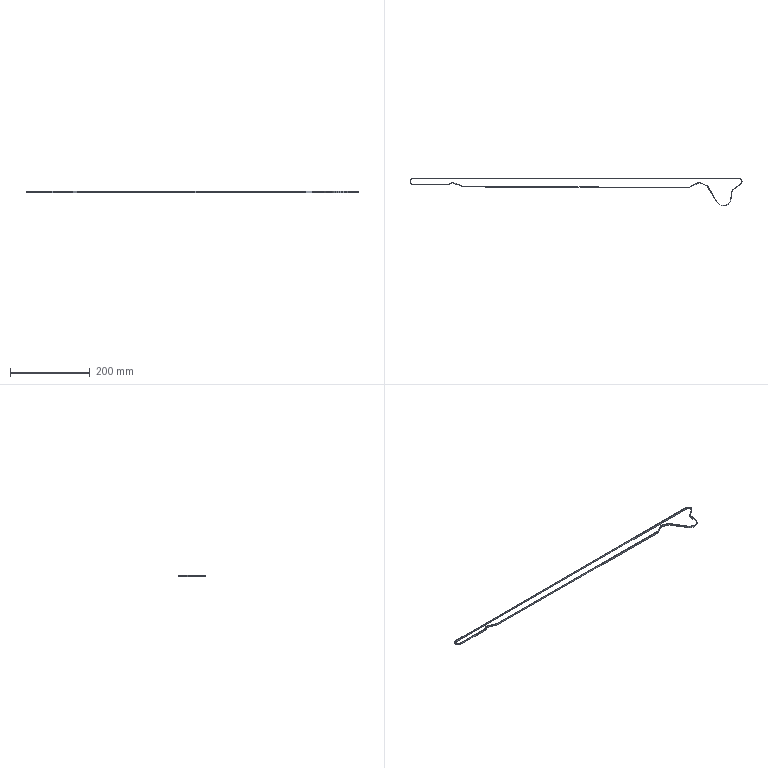Part | STEP file | Belt | 1 solid | 40 faces | box 833 x 69.5 x 4 mm | volume 6996 mm3 | cylinder 20 | plane 20 | commonest cylinder face diameters 17 x9 15 x6 19 x3 36 x1 38 x1